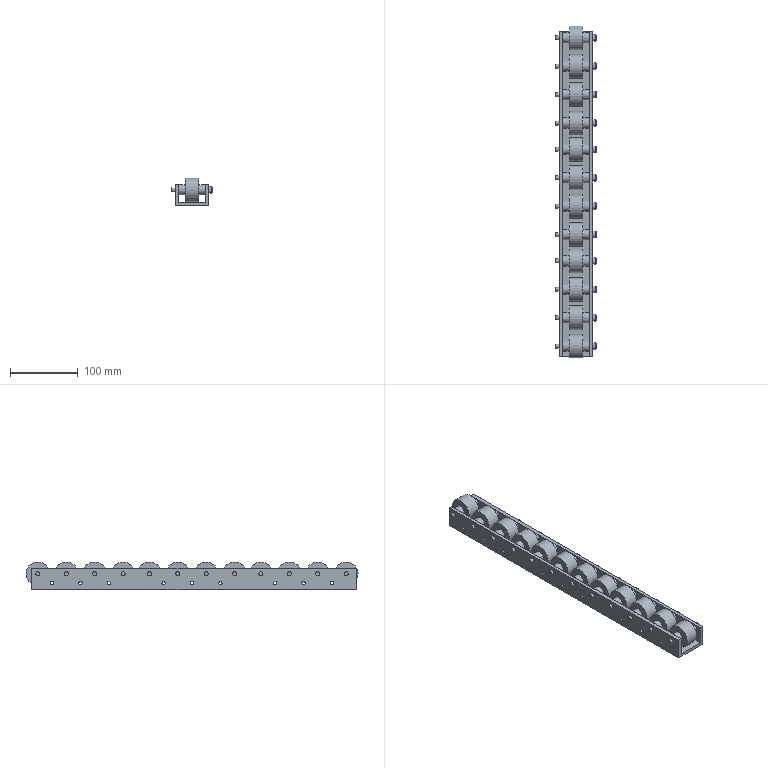Part | NX | features solid 2 | 1 solid | 148 faces | box 60 x 491 x 41.5 mm | volume 527384 mm3 | cylinder 78 | plane 58 | cone 12 | commonest cylinder face diameters 15 x24 5 x18 6 x12 10 x12 35 x12